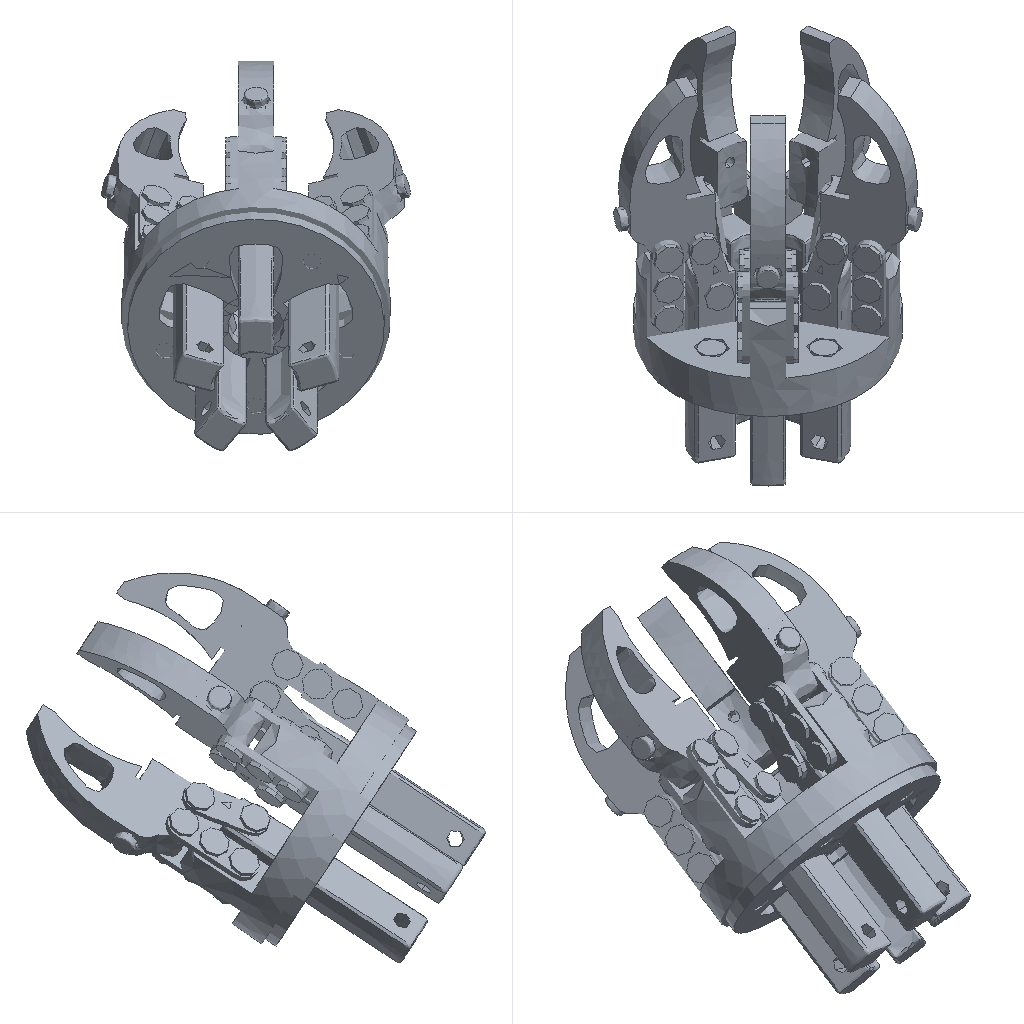Simulation study | ansys workbench
Set-up summary:
category,name,step,type,value,unit,region
solver,ansys_workbench
units,mm-N-s-tonne (MPa),,stated,"/units,MPA"
analysis,LS1,,static
load_step,LS1,LS1,static,nsubst=1; time=1
mesh,nodes,,,68074
mesh,elements,,,47218
element_type,SOLID187,,,29436
element_type,TARGE170,,,8195
element_type,CONTA174,,,8195
element_type,SURF154,,,970
element_type,SOLID186,,,422
material,Structural Steel,,E,200000,tonne s^-2 mm^-1
material,Structural Steel,,nu,0.3
material,Structural Steel,,density,7.85e-09,tonne mm^-3
material,Structural Steel,,conductivity,60.5,tonne mm s^-3 C^-1
material,Structural Steel,,specific_heat,4.34e+08,mm^2 s^-2 C^-1
material,Structural Steel,,cte,1.2e-05,C^-1
material,Structural Steel,,permeability,10000
material,Structural Steel,,resistivity,0.00017,ohm mm
load,Define Force Using Surface Effect Elements,LS1,surface-effect pres face 1,-6.57195e-16,,SURF154 #340
load,Define Force Using Surface Effect Elements,LS1,surface-effect pres face 2,-0.55,,SURF154 #340
load,Define Force Using Surface Effect Elements,LS1,surface-effect pres face 3,-0.3598,,SURF154 #340
load,Define Force Using Surface Effect Elements,LS1,surface-effect pres face 1,-0.07268,,SURF154 #341
load,Define Force Using Surface Effect Elements,LS1,surface-effect pres face 2,0.1224,,SURF154 #341
load,Define Force Using Surface Effect Elements,LS1,surface-effect pres face 3,-0.1872,,SURF154 #341
bc,Fixed Supports,model,fixed,[dofs=ALL],,_FIXEDSU
contact,Contact Region,,bonded (always),element=CONTA174
contact,Contact Region 2,,bonded (always),element=CONTA174
contact,Contact Region 3,,bonded (always),element=CONTA174
contact,Contact Region 4,,bonded (always),element=CONTA174
contact,Contact Region 5,,bonded (always),element=CONTA174
contact,Contact Region 6,,bonded (always),element=CONTA174
contact,Contact Region 7,,bonded (always),element=CONTA174
contact,Contact Region 8,,bonded (always),element=CONTA174
contact,Contact Region 9,,bonded (always),element=CONTA174
contact,Contact Region 10,,bonded (always),element=CONTA174
contact,Contact Region 11,,bonded (always),element=CONTA174
contact,Contact Region 12,,bonded (always),element=CONTA174
contact,Contact Region 13,,bonded (always),element=CONTA174
contact,Contact Region 14,,bonded (always),element=CONTA174
contact,Contact Region 15,,bonded (always),element=CONTA174
contact,Contact Region 16,,bonded (always),element=CONTA174
contact,Contact Region 17,,bonded (always),element=CONTA174
contact,Contact Region 18,,bonded (always),element=CONTA174
contact,Contact Region 19,,bonded (always),element=CONTA174
contact,Contact Region 20,,bonded (always),element=CONTA174
contact,Contact Region 21,,bonded (always),element=CONTA174
contact,Contact Region 22,,bonded (always),element=CONTA174
contact,Contact Region 23,,bonded (always),element=CONTA174
contact,Contact Region 24,,bonded (always),element=CONTA174
contact,Contact Region 25,,bonded (always),element=CONTA174
contact,Contact Region 26,,bonded (always),element=CONTA174
contact,Contact Region 27,,bonded (always),element=CONTA174
contact,Contact Region 28,,bonded (always),element=CONTA174
contact,Contact Region 29,,bonded (always),element=CONTA174
contact,Contact Region 30,,bonded (always),element=CONTA174
contact,Contact Region 31,,bonded (always),element=CONTA174
contact,Contact Region 32,,bonded (always),element=CONTA174
contact,Contact Region 33,,bonded (always),element=CONTA174
contact,Contact Region 34,,bonded (always),element=CONTA174
contact,Contact Region 35,,bonded (always),element=CONTA174
contact,Contact Region 36,,bonded (always),element=CONTA174
contact,Contact Region 37,,bonded (always),element=CONTA174
contact,Contact Region 38,,bonded (always),element=CONTA174
contact,Contact Region 39,,bonded (always),element=CONTA174
contact,Contact Region 40,,bonded (always),element=CONTA174
contact,Contact Region 41,,bonded (always),element=CONTA174
contact,Contact Region 42,,bonded (always),element=CONTA174
contact,Contact Region 43,,bonded (always),element=CONTA174
contact,Contact Region 44,,bonded (always),element=CONTA174
contact,Contact Region 45,,bonded (always),element=CONTA174
contact,Contact Region 46,,bonded (always),element=CONTA174
contact,Contact Region 47,,bonded (always),element=CONTA174
contact,Contact Region 48,,bonded (always),element=CONTA174
contact,Contact Region 49,,bonded (always),element=CONTA174
contact,Contact Region 50,,bonded (always),element=CONTA174
contact,Contact Region 51,,bonded (always),element=CONTA174
contact,Contact Region 52,,bonded (always),element=CONTA174
contact,Contact Region 53,,bonded (always),element=CONTA174
contact,Contact Region 54,,bonded (always),element=CONTA174
contact,Contact Region 55,,bonded (always),element=CONTA174
contact,Contact Region 56,,bonded (always),element=CONTA174
contact,Contact Region 57,,bonded (always),element=CONTA174
contact,Contact Region 58,,bonded (always),element=CONTA174
contact,Contact Region 59,,bonded (always),element=CONTA174
contact,Contact Region 60,,bonded (always),element=CONTA174
contact,Contact Region 61,,bonded (always),element=CONTA174
contact,Contact Region 62,,bonded (always),element=CONTA174
contact,Contact Region 63,,bonded (always),element=CONTA174
contact,Contact Region 64,,bonded (always),element=CONTA174
contact,Contact Region 65,,bonded (always),element=CONTA174
contact,Contact Region 66,,bonded (always),element=CONTA174
contact,Contact Region 67,,bonded (always),element=CONTA174
contact,Contact Region 68,,bonded (always),element=CONTA174
contact,Contact Region 69,,bonded (always),element=CONTA174
contact,Contact Region 70,,bonded (always),element=CONTA174
contact,Contact Region 71,,bonded (always),element=CONTA174
contact,Contact Region 72,,bonded (always),element=CONTA174
contact,Contact Region 73,,bonded (always),element=CONTA174
contact,Contact Region 74,,bonded (always),element=CONTA174
contact,Contact Region 75,,bonded (always),element=CONTA174
contact,Contact Region 76,,bonded (always),element=CONTA174
contact,Contact Region 77,,bonded (always),element=CONTA174
contact,Contact Region 78,,bonded (always),element=CONTA174
contact,Contact Region 79,,bonded (always),element=CONTA174
contact,Contact Region 80,,bonded (always),element=CONTA174
contact,Contact Region 81,,bonded (always),element=CONTA174
contact,Contact Region 82,,bonded (always),element=CONTA174
contact,Contact Region 83,,bonded (always),element=CONTA174
contact,Contact Region 84,,bonded (always),element=CONTA174
contact,Contact Region 85,,bonded (always),element=CONTA174
contact,Contact Region 86,,bonded (always),element=CONTA174
contact,Contact Region 87,,bonded (always),element=CONTA174
contact,Contact Region 88,,bonded (always),element=CONTA174
contact,Contact Region 89,,bonded (always),element=CONTA174
contact,Contact Region 90,,bonded (always),element=CONTA174
contact,Contact Region 91,,bonded (always),element=CONTA174
contact,Contact Region 92,,bonded (always),element=CONTA174
contact,Contact Region 93,,bonded (always),element=CONTA174
contact,Contact Region 94,,bonded (always),element=CONTA174
contact,Contact Region 95,,bonded (always),element=CONTA174
contact,Contact Region 96,,bonded (always),element=CONTA174
contact,Contact Region 97,,bonded (always),element=CONTA174
contact,Contact Region 98,,bonded (always),element=CONTA174
contact,Contact Region 99,,bonded (always),element=CONTA174
contact,Contact Region 100,,bonded (always),element=CONTA174
contact,Contact Region 101,,bonded (always),element=CONTA174
contact,Contact Region 102,,bonded (always),element=CONTA174
contact,Contact Region 103,,bonded (always),element=CONTA174
contact,Contact Region 104,,bonded (always),element=CONTA174
contact,Contact Region 105,,bonded (always),element=CONTA174
contact,Contact Region 106,,bonded (always),element=CONTA174
contact,Contact Region 107,,bonded (always),element=CONTA174
contact,Contact Region 108,,bonded (always),element=CONTA174
contact,Contact Region 109,,bonded (always),element=CONTA174
contact,Contact Region 110,,bonded (always),element=CONTA174
contact,Contact Region 111,,bonded (always),element=CONTA174
contact,Contact Region 112,,bonded (always),element=CONTA174
contact,Contact Region 113,,bonded (always),element=CONTA174
contact,Contact Region 114,,bonded (always),element=CONTA174
contact,Contact Region 115,,bonded (always),element=CONTA174
contact,Contact Region 116,,bonded (always),element=CONTA174
contact,Contact Region 117,,bonded (always),element=CONTA174
contact,Contact Region 118,,bonded (always),element=CONTA174
contact,Contact Region 119,,bonded (always),element=CONTA174
contact,Contact Region 120,,bonded (always),element=CONTA174
contact,Contact Region 121,,bonded (always),element=CONTA174
named_set,_FIXEDSU,,node,1903
Ansys APDL input file, long lists of numbers shortened:
/batch
/config,noeldb,1     ! force off writing results to database
*get,_wallstrt,active,,time,wall
! ANSYS input file written by Workbench version 2022 R1
! File used for geometry attach:
/title,wbnew--____ (A5)
! ****** Begin Custom Load Command Snippet ******
/COM, ACT Extensions:
/COM,     LSDYNA, 2021.1
/COM,
! ****** End   Custom Load Command Snippet ******
*DIM,_wb_ProjectScratch_dir,string,248
_wb_ProjectScratch_dir(1) = ''
*DIM,_wb_SolverFiles_dir,string,248
_wb_SolverFiles_dir(1) = ''
*DIM,_wb_userfiles_dir,string,248
_wb_userfiles_dir(1) = ''
/com,--- Data in consistent NMM units. See Solving Units in the help system for more information.
/units,MPA
/nopr
/wb,file,start              !  signify a WB generated input file
/prep7
! Turn off shape checking because checks already performed inside WB mesher.
! See help system for more information.
SHPP,OFF,,NOWARN
/nolist
etcon,set             ! allow ANSYS to choose best KEYOP's for 180x elements, resets any applicable keyopt to MAPDL defaults
/com,*********** Nodes for the whole assembly ***********
nblock,3,,74881
(1i9,3e20.9e3)
        1    -1.013145392E+02     1.680263990E+01     9.745129559E+02
! (68073 more lines like these left out)
-1
/wb,elem,start            !  set before creation of elements
/com,*********** Elements for Body 1 "__|NONE" ***********
et,1,187
eblock,19,solid,,560
(19i9)
        1        1        1        1        0        0        0        0       10        0    22393    52929    53128    52932    53062    53237    53256    53227    53231
! (1119 more lines like these left out)
-1
/com,*********** Elements for Body 2 "___|NONE" ***********
et,2,187
eblock,19,solid,,352
(19i9)
        2        2        2        2        0        0        0        0       10        0     2070     4821     4826     4918     4909     5169     5208     5175     5174
! (703 more lines like these left out)
-1
/com,*********** Elements for Body 3 "____|NONE" ***********
et,3,187
eblock,19,solid,,645
(19i9)
        3        3        3        3        0        0        0        0       10        0    18368    42740    42897    42874    42887    43404    43942    43400    43402
! (1289 more lines like these left out)
-1
/com,*********** Elements for Body 4 "__|NONE" ***********
et,4,186
keyo,4,2,1          ! set full integration on SOLID186
eblock,19,solid,,132
(19i9)
        4        4        4        4        0        0        0        0       20        0     6682    14978    15119    15120    15011    15045    15290    15291    15012
! (263 more lines like these left out)
-1
/com,*********** Elements for Body 5 "___|NONE" ***********
et,5,187
eblock,19,solid,,177
(19i9)
        5        5        5        5        0        0        0        0       10        0     1362     3160     3190     3162     3163     3429     3440     3424     3425
! (353 more lines like these left out)
-1
! (92 more sections like these left out)
/wb,elem,end               !  done creating elements
/com,*********** Send User Defined Coordinate System(s) ***********
csys,0
toffst,273.15,  ! Temperature offset from absolute zero
/com,*********** Set Reference Temperature ***********
tref,22.
/wb,mat,start              !  starting to send materials
/com,*********** Send Materials ***********
Temperature = 'TEMP' ! Temperature
MP,DENS,1,7.85e-09,	! tonne mm^-3
MP,ALPX,1,1.2e-05,	! C^-1
MP,C,1,434000000,	! mm^2 s^-2 C^-1
MP,KXX,1,60.5,	! tonne mm s^-3 C^-1
MP,RSVX,1,0.00017,	! ohm mm
MP,EX,1,200000,	! tonne s^-2 mm^-1
MP,NUXY,1,0.3,
MP,MURX,1,10000,
Temperature = 'TEMP' ! Temperature
MP,DENS,2,7.85e-09,	! tonne mm^-3
MP,ALPX,2,1.2e-05,	! C^-1
MP,C,2,434000000,	! mm^2 s^-2 C^-1
MP,KXX,2,60.5,	! tonne mm s^-3 C^-1
MP,RSVX,2,0.00017,	! ohm mm
MP,EX,2,200000,	! tonne s^-2 mm^-1
MP,NUXY,2,0.3,
MP,MURX,2,10000,
Temperature = 'TEMP' ! Temperature
MP,DENS,3,7.85e-09,	! tonne mm^-3
MP,ALPX,3,1.2e-05,	! C^-1
MP,C,3,434000000,	! mm^2 s^-2 C^-1
MP,KXX,3,60.5,	! tonne mm s^-3 C^-1
MP,RSVX,3,0.00017,	! ohm mm
MP,EX,3,200000,	! tonne s^-2 mm^-1
MP,NUXY,3,0.3,
MP,MURX,3,10000,
Temperature = 'TEMP' ! Temperature
MP,DENS,4,7.85e-09,	! tonne mm^-3
MP,ALPX,4,1.2e-05,	! C^-1
MP,C,4,434000000,	! mm^2 s^-2 C^-1
MP,KXX,4,60.5,	! tonne mm s^-3 C^-1
MP,RSVX,4,0.00017,	! ohm mm
MP,EX,4,200000,	! tonne s^-2 mm^-1
MP,NUXY,4,0.3,
MP,MURX,4,10000,
Temperature = 'TEMP' ! Temperature
MP,DENS,5,7.85e-09,	! tonne mm^-3
MP,ALPX,5,1.2e-05,	! C^-1
MP,C,5,434000000,	! mm^2 s^-2 C^-1
MP,KXX,5,60.5,	! tonne mm s^-3 C^-1
MP,RSVX,5,0.00017,	! ohm mm
MP,EX,5,200000,	! tonne s^-2 mm^-1
MP,NUXY,5,0.3,
MP,MURX,5,10000,
Temperature = 'TEMP' ! Temperature
MP,DENS,6,7.85e-09,	! tonne mm^-3
MP,ALPX,6,1.2e-05,	! C^-1
MP,C,6,434000000,	! mm^2 s^-2 C^-1
MP,KXX,6,60.5,	! tonne mm s^-3 C^-1
MP,RSVX,6,0.00017,	! ohm mm
MP,EX,6,200000,	! tonne s^-2 mm^-1
MP,NUXY,6,0.3,
MP,MURX,6,10000,
Temperature = 'TEMP' ! Temperature
MP,DENS,7,7.85e-09,	! tonne mm^-3
MP,ALPX,7,1.2e-05,	! C^-1
MP,C,7,434000000,	! mm^2 s^-2 C^-1
MP,KXX,7,60.5,	! tonne mm s^-3 C^-1
MP,RSVX,7,0.00017,	! ohm mm
MP,EX,7,200000,	! tonne s^-2 mm^-1
MP,NUXY,7,0.3,
MP,MURX,7,10000,
Temperature = 'TEMP' ! Temperature
MP,DENS,8,7.85e-09,	! tonne mm^-3
MP,ALPX,8,1.2e-05,	! C^-1
MP,C,8,434000000,	! mm^2 s^-2 C^-1
MP,KXX,8,60.5,	! tonne mm s^-3 C^-1
MP,RSVX,8,0.00017,	! ohm mm
MP,EX,8,200000,	! tonne s^-2 mm^-1
MP,NUXY,8,0.3,
MP,MURX,8,10000,
Temperature = 'TEMP' ! Temperature
MP,DENS,9,7.85e-09,	! tonne mm^-3
MP,ALPX,9,1.2e-05,	! C^-1
MP,C,9,434000000,	! mm^2 s^-2 C^-1
MP,KXX,9,60.5,	! tonne mm s^-3 C^-1
MP,RSVX,9,0.00017,	! ohm mm
MP,EX,9,200000,	! tonne s^-2 mm^-1
! (794 more lines like these left out)
/wb,mat,end                !  done sending materials
!************************* Model Summary ********************
!__|NONE,	结构钢,	matid,	1
!___|NONE,	结构钢,	matid,	2
!____|NONE,	结构钢,	matid,	3
! (96 more lines like these left out)
*get,_xmin,node,,mnloc,x
*get,_ymin,node,,mnloc,y
*get,_zmin,node,,mnloc,z
*get,_xmax,node,,mxloc,x
*get,_ymax,node,,mxloc,y
*get,_zmax,node,,mxloc,z
_ASMDIAG=(_xmax-_xmin)*(_xmax-_xmin)+(_ymax-_ymin)*(_ymax-_ymin)+(_zmax-_zmin)*(_zmax-_zmin)
_ASMDIAG=SQRT(_ASMDIAG)
/wb,contact,start          !  starting to send contact
/com,*********** Create Contact "接触区域" ***********
/com,            Real Constant Set For Above Contact Is 99 & 98
*set,tid,99
*set,cid,98
r,tid
r,cid
et,tid,170
et,cid,174
eblock,10,,,15
(15i9)
    52909       99       99       99        0    53007    53008    53010    53010    53677    53683    53010    53678
! (14 more lines like these left out)
-1
eblock,10,,,15
(15i9)
    52924       98       98       98        0    53007    53008    53010    53010    53677    53683    53010    53678
! (14 more lines like these left out)
-1
eblock,10,,,76
(15i9)
    52939       98       99       98        0     4824     4830     4825     4825     5190     5197     4825     5189
! (75 more lines like these left out)
-1
eblock,10,,,76
(15i9)
    53015       99       98       99        0     4824     4830     4825     4825     5190     5197     4825     5189
! (75 more lines like these left out)
-1
keyo,cid,8,2               ! auto create asymmetric contact (from Program Controlled setting)
keyo,cid,10,0              ! adjust contact stiffness each NR iteration (from Program Controlled setting)
keyo,cid,12,5              ! bonded always
keyo,cid,18,1              ! small sliding turned on by application
keyo,cid,2,0               ! augmented Lagrange (from Program Controlled setting)
keyo,cid,4,0               ! on Gauss point (from Program Controlled setting)
keyo,cid,9,1               ! ignore initial gaps/penetration
keyo,cid,7,0               ! No Prediction
rmod,tid,3,10.      ! FKN
rmod,tid,5,0.       ! ICONT
rmod,tid,6,0.       ! PINB
rmod,tid,10,0.      ! CNOF
rmod,tid,12,0.      ! FKT
rmod,tid,36,314     ! WB DSID
rmod,cid,3,10.      ! FKN
rmod,cid,5,0.       ! ICONT
rmod,cid,6,0.       ! PINB
rmod,cid,10,0.      ! CNOF
rmod,cid,12,0.      ! FKT
rmod,cid,36,314     ! WB DSID
/com,*********** Create Contact "接触区域 2" ***********
/com,            Real Constant Set For Above Contact Is 101 & 100
*set,tid,101
*set,cid,100
r,tid
r,cid
et,tid,170
et,cid,174
eblock,10,,,51
(15i9)
    53091      101      101      101        0    53015    53021    53016    53016    53717    53722    53016    53714
! (50 more lines like these left out)
-1
eblock,10,,,51
(15i9)
    53142      100      100      100        0    53015    53021    53016    53016    53717    53722    53016    53714
! (50 more lines like these left out)
-1
eblock,10,,,60
(15i9)
    53193      100      101      100        0    42812    42823    42813    42813    43688    43698    42813    43687
! (59 more lines like these left out)
-1
eblock,10,,,60
(15i9)
    53253      101      100      101        0    42812    42823    42813    42813    43688    43698    42813    43687
! (59 more lines like these left out)
-1
keyo,cid,8,2               ! auto create asymmetric contact (from Program Controlled setting)
keyo,cid,10,0              ! adjust contact stiffness each NR iteration (from Program Controlled setting)
keyo,cid,12,5              ! bonded always
keyo,cid,18,1              ! small sliding turned on by application
keyo,cid,2,0               ! augmented Lagrange (from Program Controlled setting)
keyo,cid,4,0               ! on Gauss point (from Program Controlled setting)
keyo,cid,9,1               ! ignore initial gaps/penetration
keyo,cid,7,0               ! No Prediction
rmod,tid,3,10.      ! FKN
rmod,tid,5,0.       ! ICONT
rmod,tid,6,0.       ! PINB
rmod,tid,10,0.      ! CNOF
rmod,tid,12,0.      ! FKT
rmod,tid,36,317     ! WB DSID
rmod,cid,3,10.      ! FKN
rmod,cid,5,0.       ! ICONT
rmod,cid,6,0.       ! PINB
rmod,cid,10,0.      ! CNOF
rmod,cid,12,0.      ! FKT
rmod,cid,36,317     ! WB DSID
/com,*********** Create Contact "接触区域 3" ***********
/com,            Real Constant Set For Above Contact Is 103 & 102
*set,tid,103
*set,cid,102
r,tid
r,cid
et,tid,170
et,cid,174
eblock,10,,,98
(15i9)
    53313      103      103      103        0     4798     4799     4887     4887     5017     5023     4887     5019
! (97 more lines like these left out)
-1
eblock,10,,,98
(15i9)
    53411      102      102      102        0     4798     4799     4887     4887     5017     5023     4887     5019
! (97 more lines like these left out)
-1
eblock,10,,,76
(15i9)
    53509      102      103      102        0    42711    42718    42716    42716    43192    43235    42716    43191
! (75 more lines like these left out)
-1
eblock,10,,,76
(15i9)
    53585      103      102      103        0    42711    42718    42716    42716    43192    43235    42716    43191
! (75 more lines like these left out)
-1
keyo,cid,8,2               ! auto create asymmetric contact (from Program Controlled setting)
keyo,cid,10,0              ! adjust contact stiffness each NR iteration (from Program Controlled setting)
keyo,cid,12,5              ! bonded always
keyo,cid,18,1              ! small sliding turned on by application
keyo,cid,2,0               ! augmented Lagrange (from Program Controlled setting)
keyo,cid,4,0               ! on Gauss point (from Program Controlled setting)
keyo,cid,9,1               ! ignore initial gaps/penetration
keyo,cid,7,0               ! No Prediction
rmod,tid,3,10.      ! FKN
rmod,tid,5,0.       ! ICONT
rmod,tid,6,0.       ! PINB
rmod,tid,10,0.      ! CNOF
rmod,tid,12,0.      ! FKT
rmod,tid,36,320     ! WB DSID
rmod,cid,3,10.      ! FKN
rmod,cid,5,0.       ! ICONT
rmod,cid,6,0.       ! PINB
rmod,cid,10,0.      ! CNOF
rmod,cid,12,0.      ! FKT
rmod,cid,36,320     ! WB DSID
/com,*********** Create Contact "接触区域 4" ***********
/com,            Real Constant Set For Above Contact Is 105 & 104
*set,tid,105
*set,cid,104
r,tid
r,cid
et,tid,170
et,cid,174
eblock,10,,,25
(15i9)
    53661      105      105      105        0    42681    42827    42778    42778    43015    43568    42778    43012
! (24 more lines like these left out)
-1
eblock,10,,,25
(15i9)
    53686      104      104      104        0    42681    42827    42778    42778    43015    43568    42778    43012
! (24 more lines like these left out)
-1
eblock,10,,,20
(15i9)
    53711      104      105      104        0    31581    31605    31656    31656    31697    31855    31656    31702
! (19 more lines like these left out)
-1
eblock,10,,,20
(15i9)
    53731      105      104      105        0    31581    31605    31656    31656    31697    31855    31656    31702
! (19 more lines like these left out)
-1
keyo,cid,8,2               ! auto create asymmetric contact (from Program Controlled setting)
keyo,cid,10,0              ! adjust contact stiffness each NR iteration (from Program Controlled setting)
keyo,cid,12,5              ! bonded always
keyo,cid,18,1              ! small sliding turned on by application
keyo,cid,2,0               ! augmented Lagrange (from Program Controlled setting)
keyo,cid,4,0               ! on Gauss point (from Program Controlled setting)
keyo,cid,9,1               ! ignore initial gaps/penetration
keyo,cid,7,0               ! No Prediction
rmod,tid,3,10.      ! FKN
rmod,tid,5,0.       ! ICONT
rmod,tid,6,0.       ! PINB
rmod,tid,10,0.      ! CNOF
rmod,tid,12,0.      ! FKT
rmod,tid,36,323     ! WB DSID
rmod,cid,3,10.      ! FKN
rmod,cid,5,0.       ! ICONT
rmod,cid,6,0.       ! PINB
rmod,cid,10,0.      ! CNOF
rmod,cid,12,0.      ! FKT
rmod,cid,36,323     ! WB DSID
/com,*********** Create Contact "接触区域 5" ***********
/com,            Real Constant Set For Above Contact Is 107 & 106
*set,tid,107
*set,cid,106
r,tid
r,cid
et,tid,170
et,cid,174
eblock,10,,,20
(15i9)
    53751      107      107      107        0    42670    42784    42828    42828    42922    43584    42828    42927
! (19 more lines like these left out)
-1
eblock,10,,,20
(15i9)
    53771      106      106      106        0    42670    42784    42828    42828    42922    43584    42828    42927
! (19 more lines like these left out)
-1
eblock,10,,,12
(15i9)
    53791      106      107      106        0    37512    37518    37517    37509    37634    37649    37625    37624
! (11 more lines like these left out)
-1
eblock,10,,,12
(15i9)
    53803      107      106      107        0    37512    37518    37517    37509    37634    37649    37625    37624
! (11 more lines like these left out)
-1
keyo,cid,8,2               ! auto create asymmetric contact (from Program Controlled setting)
keyo,cid,10,0              ! adjust contact stiffness each NR iteration (from Program Controlled setting)
keyo,cid,12,5              ! bonded always
keyo,cid,18,1              ! small sliding turned on by application
keyo,cid,2,0               ! augmented Lagrange (from Program Controlled setting)
keyo,cid,4,0               ! on Gauss point (from Program Controlled setting)
keyo,cid,9,1               ! ignore initial gaps/penetration
keyo,cid,7,0               ! No Prediction
rmod,tid,3,10.      ! FKN
rmod,tid,5,0.       ! ICONT
rmod,tid,6,0.       ! PINB
rmod,tid,10,0.      ! CNOF
rmod,tid,12,0.      ! FKT
rmod,tid,36,326     ! WB DSID
rmod,cid,3,10.      ! FKN
rmod,cid,5,0.       ! ICONT
rmod,cid,6,0.       ! PINB
rmod,cid,10,0.      ! CNOF
rmod,cid,12,0.      ! FKT
rmod,cid,36,326     ! WB DSID
! (116 more sections like these left out)
/wb,contact,end            !  done creating contacts
/golist
/wb,load,start             !  starting to send loads
/com,*********** Fixed Supports ***********
CMBLOCK,_FIXEDSU,NODE,     1903
(8i10)
      6414      6415      6416      6417      6418      6419      6420      6421
! (237 more lines like these left out)
cmsel,s,_FIXEDSU
d,all,all
nsel,all
/com,*********** Define Force Using Surface Effect Elements ***********
local,12,0,0.,0.,0.,0.,0.,0.
csys,0
et,340,154
eblock,10,,,810
(15i9)
    69299      340      340      340       12    22566    22862    22758    22758    24216    25048    22758    24211
! (809 more lines like these left out)
-1
esel,s,type,,340
keyop,340,2,1                ! Apply load in local coordinate system
keyop,340,7,1                ! Use original area so load is constant in large deformation
esel,all
/com,*********** Define Force Using Surface Effect Elements ***********
local,13,0,0.,0.,0.,0.,0.,0.
csys,0
et,341,154
eblock,10,,,160
(15i9)
    70109      341      341      341       13    60285    60291    60287    60287    60624    60641    60287    60623
! (159 more lines like these left out)
-1
esel,s,type,,341
keyop,341,2,1                ! Apply load in local coordinate system
keyop,341,7,1                ! Use original area so load is constant in large deformation
esel,all
/gst,on,on
fini
*get,_numnode,node,0,count
*get,_numelem,elem,0,count
*get, _MAXELEMNUM, elem, 0, NUM, MAX
*get, _MAXNODENUM, node, 0, NUM, MAX
*get, _MAXELEMTYPE, etyp, 0, NUM, MAX
*get, _MAXREALCONST, real, 0, NUM, MAX
/go
/wb,load,end               !  done creating loads
/com,--- Number of total nodes = %_numnode%
/com,--- Number of contact elements = 17360
/com,--- Number of spring elements = 0
/com,--- Number of bearing elements = 0
/com,--- Number of solid elements = 29858
/com,--- Number of condensed parts = 0
/com,--- Number of total elements = %_numelem%
*get,_wallbsol,active,,time,wall
/com,****************************************************************************
/com,*************************    SOLUTION       ********************************
/com,****************************************************************************
/solu
antype,0                   ! static analysis
_thickRatio=0.103   ! Ratio of thick parts in the model
eqsl,sparse,,,,,1
cntr,print,1               ! print out contact info and also make no initial contact an error
cntr,out,yes               ! write contact output to file.cmn due to many contact pairs present
dmpoption,emat,no             ! Don't combine emat file for DANSYS
dmpoption,esav,no             ! Don't combine esav file for DANSYS
nldiag,cont,iter           ! print out contact info each equilibrium iteration
rescontrol,,none                 ! Do not keep any restart files
/com,****************************************************
/com,******************* SOLVE FOR LS 1 OF 1 ****************
esel,s,type,,340
nsle
sfe,all,1,pres,1,-6.5719498526903e-016
sfe,all,2,pres,1,-0.55
sfe,all,3,pres,1,-0.3598
esel,s,type,,341
nsle
sfe,all,1,pres,1,-7.26760108341931e-002
sfe,all,2,pres,1,0.1224
sfe,all,3,pres,1,-0.1872
nsel,all
esel,all
/nopr
/gopr
nsub,1,1,1
time,1.
outres,erase
outres,all,none
outres,nsol,all,
outres,rsol,all
outres,eangl,all
outres,etmp,all
outres,veng,all
outres,strs,all,
outres,epel,all,
outres,eppl,all,
outres,cont,all,
! *********** WB SOLVE COMMAND ***********
! check interactive state
*get,ANSINTER_,active,,int
*if,ANSINTER_,ne,0,then
/eof
*endif
solve
/com *************** Write FE CONNECTORS *********
CEWRITE,file,ce,,INTE
/com,****************************************************
/com,*************** FINISHED SOLVE FOR LS 1 *************
*get,_wallasol,active,,time,wall
/nopr
*get,_numnode,node,0,count
*get,_numelem,elem,0,count
*get, _MAXELEMNUM, elem, 0, NUM, MAX
*get, _MAXNODENUM, node, 0, NUM, MAX,,,INTERNAL
*get, _MAXELEMTYPE, etyp, 0, NUM, MAX
*get, _MAXREALCONST, real, 0, NUM, MAX
/gopr
/post1
xmlo,ENCODING,ISO-8859-1
xmlo,parm
/xml,parm,xml
fini
/gopr
*get,_walldone,active,,time,wall
_preptime=(_wallbsol-_wallstrt)*3600
_solvtime=(_wallasol-_wallbsol)*3600
_posttime=(_walldone-_wallasol)*3600
_totaltim=(_walldone-_wallstrt)*3600
*get,_dlbratio,active,0,solu,dlbr
*get,_combtime,active,0,solu,comb
*get,_ssmode,active,0,solu,ssmm
*get,_ndofs,active,0,solu,ndof
*get,_sol_end_time,active,0,set,time
*if,_sol_end_time,eq,1.,then
/fclean				!clean distributed files
*endif
/com,--- Total number of nodes = %_numnode%
/com,--- Total number of elements = %_numelem%
/com,--- Element load balance ratio = %_dlbratio%
/com,--- Time to combine distributed files = %_combtime%
/com,--- Sparse memory mode = %_ssmode%
/com,--- Number of DOF = %_ndofs%
/wb,file,end               ! done with WB generated input
Results summary:
result,analyses[0].index,,,1
result,analyses[0].system,,,SYS
result,analyses[0].deck,,,deck.dat
result,analyses[0].solve_status,,,completed
result,analyses[0].analysis_type,,,static
result,analyses[0].physics,,,mechanical
result,analyses[0].unit_system,,,"NMM: mm, ton, N, s, mV, mA, degC"
result,analyses[0].n_sets,,,1
result,analyses[0].load_steps[0].set,set=1,,1
result,analyses[0].load_steps[0].time_or_freq,set=1,,1
result,analyses[0].load_steps[0].max_displacement_magnitude,set=1,,0.0007793
result,analyses[0].load_steps[0].max_von_mises_nodal,set=1,,28.435
result,analyses[0].load_steps[0].reaction_force_sum_xyz[1],set=1,,154.508
result,analyses[0].load_steps[0].reaction_force_sum_xyz[2],set=1,,3923.96
result,analyses[0].load_steps[0].reaction_force_sum_xyz[3],set=1,,3135.07